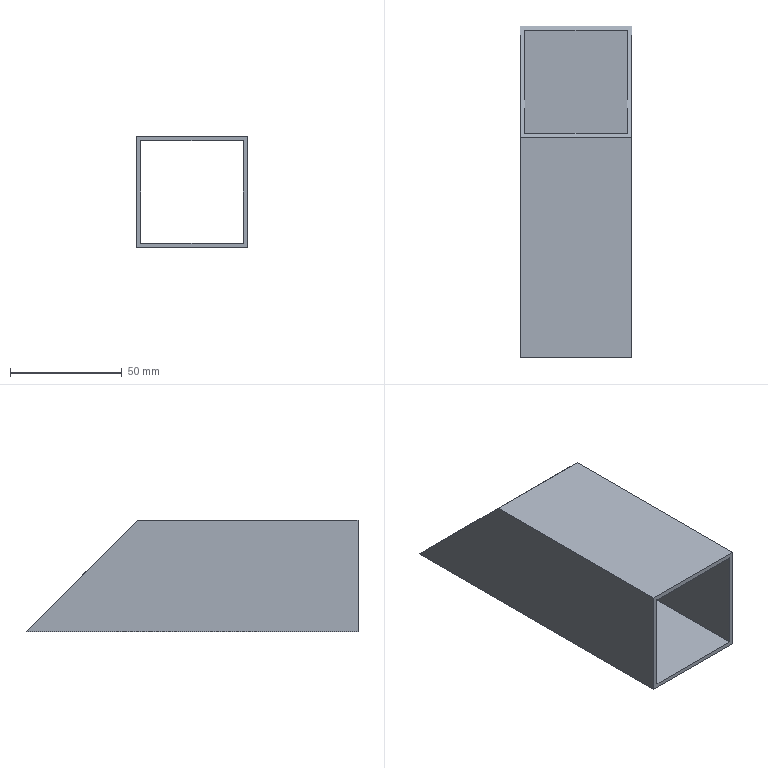Part | SolidWorks | features BaseBody 1 | 1 solid | 10 faces | box 50 x 148.338 x 50 mm | volume 47362 mm3 | plane 10
STEP:
#1=CARTESIAN_POINT('',(25.,0.,-25.));
#2=VERTEX_POINT('',#1);
#3=CARTESIAN_POINT('',(-25.,0.,-25.));
#4=VERTEX_POINT('',#3);
#5=CARTESIAN_POINT('',(-25.,0.,-25.));
#6=DIRECTION('',(-1.,0.,0.));
#7=VECTOR('',#6,1000.);
#8=LINE('',#5,#7);
#9=EDGE_CURVE('',#2,#4,#8,.T.);
#10=ORIENTED_EDGE('',*,*,#9,.T.);
#11=CARTESIAN_POINT('',(-25.,148.338,-25.));
#12=VERTEX_POINT('',#11);
#13=CARTESIAN_POINT('',(-25.,150.,-25.));
#14=DIRECTION('',(0.,1.,0.));
#15=VECTOR('',#14,1000.);
#16=LINE('',#13,#15);
#17=EDGE_CURVE('',#4,#12,#16,.T.);
#18=ORIENTED_EDGE('',*,*,#17,.T.);
#19=CARTESIAN_POINT('',(25.,148.338,-25.));
#20=VERTEX_POINT('',#19);
#21=CARTESIAN_POINT('',(-25.,148.338,-25.));
#22=DIRECTION('',(1.,0.,0.));
#23=VECTOR('',#22,1000.);
#24=LINE('',#21,#23);
#25=EDGE_CURVE('',#12,#20,#24,.T.);
#26=ORIENTED_EDGE('',*,*,#25,.T.);
#27=CARTESIAN_POINT('',(25.,150.,-25.));
#28=DIRECTION('',(0.,-1.,0.));
#29=VECTOR('',#28,1000.);
#30=LINE('',#27,#29);
#31=EDGE_CURVE('',#20,#2,#30,.T.);
#32=ORIENTED_EDGE('',*,*,#31,.T.);
#33=EDGE_LOOP('',(#10,#18,#26,#32));
#34=FACE_OUTER_BOUND('',#33,.T.);
#35=CARTESIAN_POINT('',(-25.,150.,-25.));
#36=DIRECTION('',(0.,0.,-1.));
#37=DIRECTION('',(-1.,0.,0.));
#38=AXIS2_PLACEMENT_3D('',#35,#36,#37);
#39=PLANE('',#38);
#40=ADVANCED_FACE('',(#34),#39,.T.);
#41=CARTESIAN_POINT('',(-25.,0.,25.));
#42=VERTEX_POINT('',#41);
#43=CARTESIAN_POINT('',(-25.,0.,25.));
#44=DIRECTION('',(0.,0.,1.));
#45=VECTOR('',#44,1000.);
#46=LINE('',#43,#45);
#47=EDGE_CURVE('',#4,#42,#46,.T.);
#48=ORIENTED_EDGE('',*,*,#47,.T.);
#49=CARTESIAN_POINT('',(-25.,98.338,25.));
#50=VERTEX_POINT('',#49);
#51=CARTESIAN_POINT('',(-25.,150.,25.));
#52=DIRECTION('',(0.,1.,0.));
#53=VECTOR('',#52,1000.);
#54=LINE('',#51,#53);
#55=EDGE_CURVE('',#42,#50,#54,.T.);
#56=ORIENTED_EDGE('',*,*,#55,.T.);
#57=CARTESIAN_POINT('',(-25.,98.338,25.));
#58=DIRECTION('',(0.,0.7071,-0.7071));
#59=VECTOR('',#58,1000.);
#60=LINE('',#57,#59);
#61=EDGE_CURVE('',#50,#12,#60,.T.);
#62=ORIENTED_EDGE('',*,*,#61,.T.);
#63=ORIENTED_EDGE('',*,*,#17,.F.);
#64=EDGE_LOOP('',(#48,#56,#62,#63));
#65=FACE_OUTER_BOUND('',#64,.T.);
#66=CARTESIAN_POINT('',(-25.,150.,25.));
#67=DIRECTION('',(-1.,0.,0.));
#68=DIRECTION('',(0.,0.,1.));
#69=AXIS2_PLACEMENT_3D('',#66,#67,#68);
#70=PLANE('',#69);
#71=ADVANCED_FACE('',(#65),#70,.T.);
#72=CARTESIAN_POINT('',(25.,0.,25.));
#73=VERTEX_POINT('',#72);
#74=CARTESIAN_POINT('',(25.,0.,0.));
#75=DIRECTION('',(0.,0.,-1.));
#76=VECTOR('',#75,1000.);
#77=LINE('',#74,#76);
#78=EDGE_CURVE('',#73,#2,#77,.T.);
#79=ORIENTED_EDGE('',*,*,#78,.F.);
#80=CARTESIAN_POINT('',(0.,0.,25.));
#81=DIRECTION('',(1.,0.,0.));
#82=VECTOR('',#81,1000.);
#83=LINE('',#80,#82);
#84=EDGE_CURVE('',#42,#73,#83,.T.);
#85=ORIENTED_EDGE('',*,*,#84,.F.);
#86=ORIENTED_EDGE('',*,*,#47,.F.);
#87=ORIENTED_EDGE('',*,*,#9,.F.);
#88=EDGE_LOOP('',(#79,#85,#86,#87));
#89=FACE_OUTER_BOUND('',#88,.T.);
#90=CARTESIAN_POINT('',(-23.,0.,-23.));
#91=VERTEX_POINT('',#90);
#92=CARTESIAN_POINT('',(23.,0.,-23.));
#93=VERTEX_POINT('',#92);
#94=CARTESIAN_POINT('',(0.,0.,-23.));
#95=DIRECTION('',(1.,0.,0.));
#96=VECTOR('',#95,1000.);
#97=LINE('',#94,#96);
#98=EDGE_CURVE('',#91,#93,#97,.T.);
#99=ORIENTED_EDGE('',*,*,#98,.F.);
#100=CARTESIAN_POINT('',(-23.,0.,23.));
#101=VERTEX_POINT('',#100);
#102=CARTESIAN_POINT('',(-23.,0.,0.));
#103=DIRECTION('',(0.,0.,-1.));
#104=VECTOR('',#103,1000.);
#105=LINE('',#102,#104);
#106=EDGE_CURVE('',#101,#91,#105,.T.);
#107=ORIENTED_EDGE('',*,*,#106,.F.);
#108=CARTESIAN_POINT('',(23.,0.,23.));
#109=VERTEX_POINT('',#108);
#110=CARTESIAN_POINT('',(0.,0.,23.));
#111=DIRECTION('',(-1.,0.,0.));
#112=VECTOR('',#111,1000.);
#113=LINE('',#110,#112);
#114=EDGE_CURVE('',#109,#101,#113,.T.);
#115=ORIENTED_EDGE('',*,*,#114,.F.);
#116=CARTESIAN_POINT('',(23.,0.,0.));
#117=DIRECTION('',(0.,0.,1.));
#118=VECTOR('',#117,1000.);
#119=LINE('',#116,#118);
#120=EDGE_CURVE('',#93,#109,#119,.T.);
#121=ORIENTED_EDGE('',*,*,#120,.F.);
#122=EDGE_LOOP('',(#99,#107,#115,#121));
#123=FACE_BOUND('',#122,.T.);
#124=CARTESIAN_POINT('',(0.,0.,0.));
#125=DIRECTION('',(0.,1.,0.));
#126=DIRECTION('',(0.,0.,1.));
#127=AXIS2_PLACEMENT_3D('',#124,#125,#126);
#128=PLANE('',#127);
#129=ADVANCED_FACE('',(#89,#123),#128,.F.);
#130=CARTESIAN_POINT('',(25.,98.338,25.));
#131=VERTEX_POINT('',#130);
#132=CARTESIAN_POINT('',(25.,98.338,25.));
#133=DIRECTION('',(0.,0.7071,-0.7071));
#134=VECTOR('',#133,1000.);
#135=LINE('',#132,#134);
#136=EDGE_CURVE('',#131,#20,#135,.T.);
#137=ORIENTED_EDGE('',*,*,#136,.F.);
#138=CARTESIAN_POINT('',(25.,150.,25.));
#139=DIRECTION('',(0.,1.,0.));
#140=VECTOR('',#139,1000.);
#141=LINE('',#138,#140);
#142=EDGE_CURVE('',#73,#131,#141,.T.);
#143=ORIENTED_EDGE('',*,*,#142,.F.);
#144=ORIENTED_EDGE('',*,*,#78,.T.);
#145=ORIENTED_EDGE('',*,*,#31,.F.);
#146=EDGE_LOOP('',(#137,#143,#144,#145));
#147=FACE_OUTER_BOUND('',#146,.T.);
#148=CARTESIAN_POINT('',(25.,150.,25.));
#149=DIRECTION('',(-1.,0.,0.));
#150=DIRECTION('',(0.,0.,1.));
#151=AXIS2_PLACEMENT_3D('',#148,#149,#150);
#152=PLANE('',#151);
#153=ADVANCED_FACE('',(#147),#152,.F.);
#154=CARTESIAN_POINT('',(-23.,100.338,23.));
#155=VERTEX_POINT('',#154);
#156=CARTESIAN_POINT('',(23.,100.338,23.));
#157=VERTEX_POINT('',#156);
#158=CARTESIAN_POINT('',(-25.01,100.338,23.));
#159=DIRECTION('',(1.,0.,0.));
#160=VECTOR('',#159,1000.);
#161=LINE('',#158,#160);
#162=EDGE_CURVE('',#155,#157,#161,.T.);
#163=ORIENTED_EDGE('',*,*,#162,.F.);
#164=CARTESIAN_POINT('',(-23.,146.338,-23.));
#165=VERTEX_POINT('',#164);
#166=CARTESIAN_POINT('',(-23.,98.338,25.));
#167=DIRECTION('',(0.,-0.7071,0.7071));
#168=VECTOR('',#167,1000.);
#169=LINE('',#166,#168);
#170=EDGE_CURVE('',#165,#155,#169,.T.);
#171=ORIENTED_EDGE('',*,*,#170,.F.);
#172=CARTESIAN_POINT('',(23.,146.338,-23.));
#173=VERTEX_POINT('',#172);
#174=CARTESIAN_POINT('',(-25.01,146.338,-23.));
#175=DIRECTION('',(-1.,0.,0.));
#176=VECTOR('',#175,1000.);
#177=LINE('',#174,#176);
#178=EDGE_CURVE('',#173,#165,#177,.T.);
#179=ORIENTED_EDGE('',*,*,#178,.F.);
#180=CARTESIAN_POINT('',(23.,98.338,25.));
#181=DIRECTION('',(0.,0.7071,-0.7071));
#182=VECTOR('',#181,1000.);
#183=LINE('',#180,#182);
#184=EDGE_CURVE('',#157,#173,#183,.T.);
#185=ORIENTED_EDGE('',*,*,#184,.F.);
#186=EDGE_LOOP('',(#163,#171,#179,#185));
#187=FACE_BOUND('',#186,.T.);
#188=CARTESIAN_POINT('',(-25.01,98.338,25.));
#189=DIRECTION('',(-1.,0.,0.));
#190=VECTOR('',#189,1000.);
#191=LINE('',#188,#190);
#192=EDGE_CURVE('',#131,#50,#191,.T.);
#193=ORIENTED_EDGE('',*,*,#192,.F.);
#194=ORIENTED_EDGE('',*,*,#136,.T.);
#195=ORIENTED_EDGE('',*,*,#25,.F.);
#196=ORIENTED_EDGE('',*,*,#61,.F.);
#197=EDGE_LOOP('',(#193,#194,#195,#196));
#198=FACE_OUTER_BOUND('',#197,.T.);
#199=CARTESIAN_POINT('',(-25.01,98.338,25.));
#200=DIRECTION('',(0.,-0.7071,-0.7071));
#201=DIRECTION('',(0.,0.7071,-0.7071));
#202=AXIS2_PLACEMENT_3D('',#199,#200,#201);
#203=PLANE('',#202);
#204=ADVANCED_FACE('',(#187,#198),#203,.F.);
#205=ORIENTED_EDGE('',*,*,#192,.T.);
#206=ORIENTED_EDGE('',*,*,#55,.F.);
#207=ORIENTED_EDGE('',*,*,#84,.T.);
#208=ORIENTED_EDGE('',*,*,#142,.T.);
#209=EDGE_LOOP('',(#205,#206,#207,#208));
#210=FACE_OUTER_BOUND('',#209,.T.);
#211=CARTESIAN_POINT('',(-25.,150.,25.));
#212=DIRECTION('',(0.,0.,-1.));
#213=DIRECTION('',(-1.,0.,0.));
#214=AXIS2_PLACEMENT_3D('',#211,#212,#213);
#215=PLANE('',#214);
#216=ADVANCED_FACE('',(#210),#215,.F.);
#217=ORIENTED_EDGE('',*,*,#120,.T.);
#218=CARTESIAN_POINT('',(23.,150.,23.));
#219=DIRECTION('',(0.,1.,0.));
#220=VECTOR('',#219,1000.);
#221=LINE('',#218,#220);
#222=EDGE_CURVE('',#109,#157,#221,.T.);
#223=ORIENTED_EDGE('',*,*,#222,.T.);
#224=ORIENTED_EDGE('',*,*,#184,.T.);
#225=CARTESIAN_POINT('',(23.,150.,-23.));
#226=DIRECTION('',(0.,-1.,0.));
#227=VECTOR('',#226,1000.);
#228=LINE('',#225,#227);
#229=EDGE_CURVE('',#173,#93,#228,.T.);
#230=ORIENTED_EDGE('',*,*,#229,.T.);
#231=EDGE_LOOP('',(#217,#223,#224,#230));
#232=FACE_OUTER_BOUND('',#231,.T.);
#233=CARTESIAN_POINT('',(23.,150.,25.));
#234=DIRECTION('',(-1.,0.,0.));
#235=DIRECTION('',(0.,0.,1.));
#236=AXIS2_PLACEMENT_3D('',#233,#234,#235);
#237=PLANE('',#236);
#238=ADVANCED_FACE('',(#232),#237,.T.);
#239=ORIENTED_EDGE('',*,*,#178,.T.);
#240=CARTESIAN_POINT('',(-23.,150.,-23.));
#241=DIRECTION('',(0.,1.,0.));
#242=VECTOR('',#241,1000.);
#243=LINE('',#240,#242);
#244=EDGE_CURVE('',#91,#165,#243,.T.);
#245=ORIENTED_EDGE('',*,*,#244,.F.);
#246=ORIENTED_EDGE('',*,*,#98,.T.);
#247=ORIENTED_EDGE('',*,*,#229,.F.);
#248=EDGE_LOOP('',(#239,#245,#246,#247));
#249=FACE_OUTER_BOUND('',#248,.T.);
#250=CARTESIAN_POINT('',(-25.,150.,-23.));
#251=DIRECTION('',(0.,0.,-1.));
#252=DIRECTION('',(-1.,0.,0.));
#253=AXIS2_PLACEMENT_3D('',#250,#251,#252);
#254=PLANE('',#253);
#255=ADVANCED_FACE('',(#249),#254,.F.);
#256=ORIENTED_EDGE('',*,*,#170,.T.);
#257=CARTESIAN_POINT('',(-23.,150.,23.));
#258=DIRECTION('',(0.,1.,0.));
#259=VECTOR('',#258,1000.);
#260=LINE('',#257,#259);
#261=EDGE_CURVE('',#101,#155,#260,.T.);
#262=ORIENTED_EDGE('',*,*,#261,.F.);
#263=ORIENTED_EDGE('',*,*,#106,.T.);
#264=ORIENTED_EDGE('',*,*,#244,.T.);
#265=EDGE_LOOP('',(#256,#262,#263,#264));
#266=FACE_OUTER_BOUND('',#265,.T.);
#267=CARTESIAN_POINT('',(-23.,150.,25.));
#268=DIRECTION('',(-1.,0.,0.));
#269=DIRECTION('',(0.,0.,1.));
#270=AXIS2_PLACEMENT_3D('',#267,#268,#269);
#271=PLANE('',#270);
#272=ADVANCED_FACE('',(#266),#271,.F.);
#273=ORIENTED_EDGE('',*,*,#114,.T.);
#274=ORIENTED_EDGE('',*,*,#261,.T.);
#275=ORIENTED_EDGE('',*,*,#162,.T.);
#276=ORIENTED_EDGE('',*,*,#222,.F.);
#277=EDGE_LOOP('',(#273,#274,#275,#276));
#278=FACE_OUTER_BOUND('',#277,.T.);
#279=CARTESIAN_POINT('',(-25.,150.,23.));
#280=DIRECTION('',(0.,0.,-1.));
#281=DIRECTION('',(-1.,0.,0.));
#282=AXIS2_PLACEMENT_3D('',#279,#280,#281);
#283=PLANE('',#282);
#284=ADVANCED_FACE('',(#278),#283,.T.);
#285=CLOSED_SHELL('',(#40,#71,#129,#153,#204,#216,#238,#255,#272,#284));
#286=MANIFOLD_SOLID_BREP('',#285);
#287=CARTESIAN_POINT('',(0.,0.,0.));
#288=DIRECTION('',(0.,0.,1.));
#289=DIRECTION('',(1.,0.,0.));
#290=AXIS2_PLACEMENT_3D('',#287,#288,#289);
#291=(LENGTH_UNIT()NAMED_UNIT(*)SI_UNIT(.MILLI.,.METRE.));
#292=UNCERTAINTY_MEASURE_WITH_UNIT(LENGTH_MEASURE(0.00001),#291,'','');
#293=(NAMED_UNIT(*)PLANE_ANGLE_UNIT()SI_UNIT($,.RADIAN.));
#294=(NAMED_UNIT(*)SI_UNIT($,.STERADIAN.)SOLID_ANGLE_UNIT());
#295=(GEOMETRIC_REPRESENTATION_CONTEXT(3)GLOBAL_UNCERTAINTY_ASSIGNED_CONTEXT((#292))GLOBAL_UNIT_ASSIGNED_CONTEXT((#291,#293,#294))REPRESENTATION_CONTEXT('',''));
#296=ADVANCED_BREP_SHAPE_REPRESENTATION('',(#286,#290),#295);